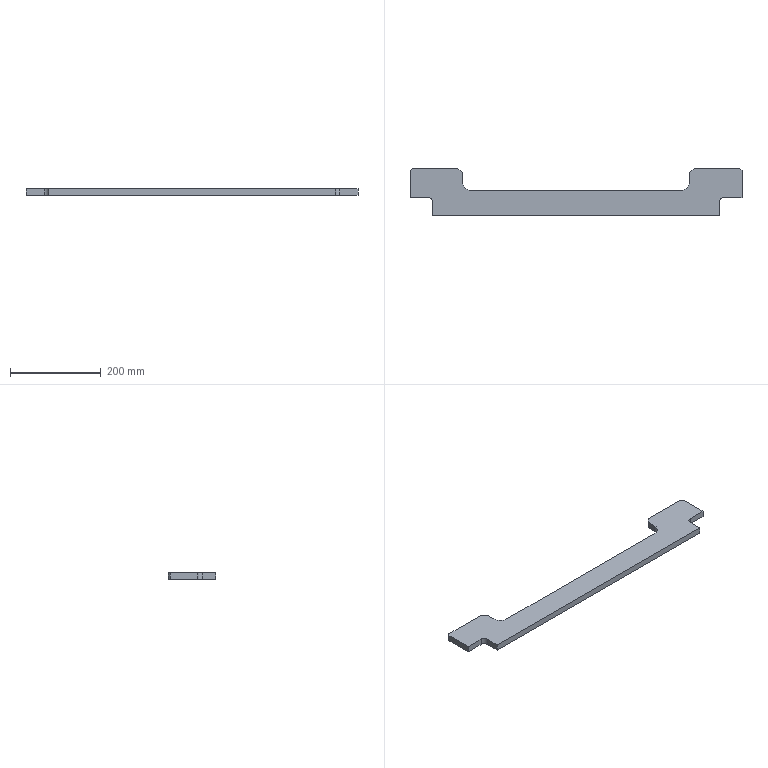Part | STEP file | Backup 2012-3-22-09 | 1 solid | 22 faces | box 730 x 105 x 14 mm | volume 668354 mm3 | plane 18 | cylinder 4 | commonest cylinder face diameters 20 x2 40 x2